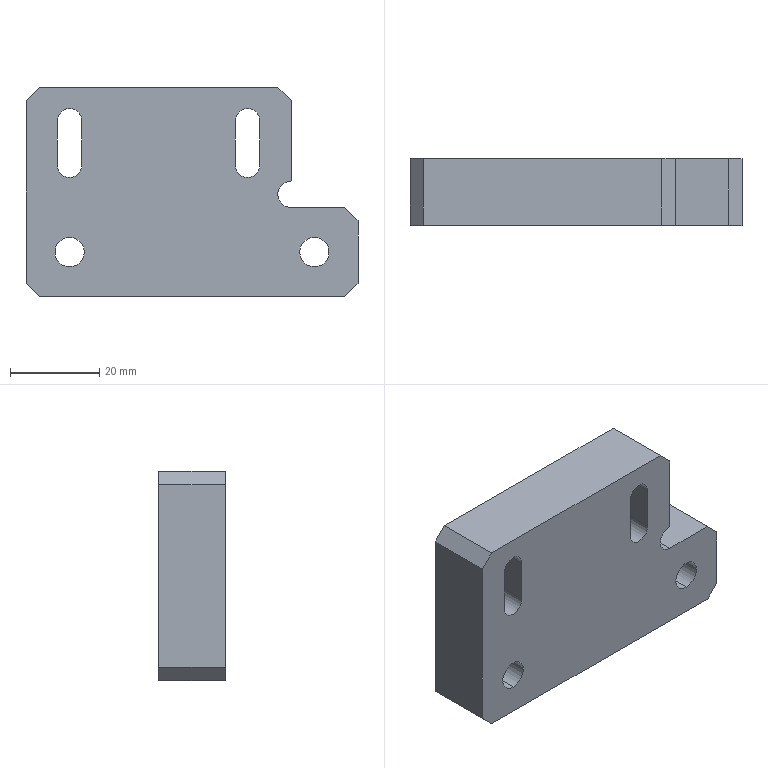Part | STEP file | front rail support plate | 1 solid | 28 faces | box 74.6 x 15 x 47 mm | volume 42579 mm3 | plane 17 | cylinder 11 | commonest cylinder face diameters 5.5 x6 6.6 x4 6 x1